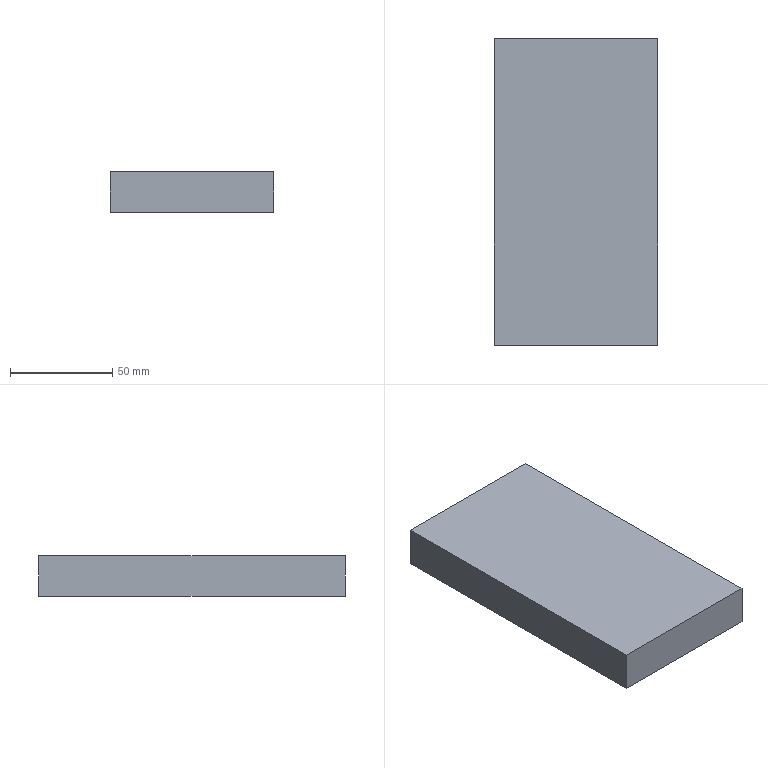Part | SolidWorks | features Extrusion 1 | 1 solid | 6 faces | box 80 x 150 x 20 mm | volume 240000 mm3 | plane 6
STEP:
#1=CARTESIAN_POINT('',(-40.,75.,0.));
#2=VERTEX_POINT('',#1);
#3=CARTESIAN_POINT('',(-40.,-75.,0.));
#4=VERTEX_POINT('',#3);
#5=CARTESIAN_POINT('',(-40.,-75.,0.));
#6=DIRECTION('',(0.,-1.,0.));
#7=VECTOR('',#6,1000.);
#8=LINE('',#5,#7);
#9=EDGE_CURVE('',#2,#4,#8,.T.);
#10=ORIENTED_EDGE('',*,*,#9,.T.);
#11=CARTESIAN_POINT('',(-40.,-75.,20.));
#12=VERTEX_POINT('',#11);
#13=CARTESIAN_POINT('',(-40.,-75.,20.));
#14=DIRECTION('',(0.,0.,-1.));
#15=VECTOR('',#14,1000.);
#16=LINE('',#13,#15);
#17=EDGE_CURVE('',#12,#4,#16,.T.);
#18=ORIENTED_EDGE('',*,*,#17,.F.);
#19=CARTESIAN_POINT('',(-40.,75.,20.));
#20=VERTEX_POINT('',#19);
#21=CARTESIAN_POINT('',(-40.,-75.,20.));
#22=DIRECTION('',(0.,-1.,0.));
#23=VECTOR('',#22,1000.);
#24=LINE('',#21,#23);
#25=EDGE_CURVE('',#20,#12,#24,.T.);
#26=ORIENTED_EDGE('',*,*,#25,.F.);
#27=CARTESIAN_POINT('',(-40.,75.,20.));
#28=DIRECTION('',(0.,0.,-1.));
#29=VECTOR('',#28,1000.);
#30=LINE('',#27,#29);
#31=EDGE_CURVE('',#20,#2,#30,.T.);
#32=ORIENTED_EDGE('',*,*,#31,.T.);
#33=EDGE_LOOP('',(#10,#18,#26,#32));
#34=FACE_OUTER_BOUND('',#33,.T.);
#35=CARTESIAN_POINT('',(-40.,-75.,20.));
#36=DIRECTION('',(1.,0.,0.));
#37=DIRECTION('',(0.,0.,-1.));
#38=AXIS2_PLACEMENT_3D('',#35,#36,#37);
#39=PLANE('',#38);
#40=ADVANCED_FACE('',(#34),#39,.F.);
#41=CARTESIAN_POINT('',(40.,-75.,0.));
#42=VERTEX_POINT('',#41);
#43=CARTESIAN_POINT('',(40.,-75.,0.));
#44=DIRECTION('',(1.,0.,0.));
#45=VECTOR('',#44,1000.);
#46=LINE('',#43,#45);
#47=EDGE_CURVE('',#4,#42,#46,.T.);
#48=ORIENTED_EDGE('',*,*,#47,.T.);
#49=CARTESIAN_POINT('',(40.,-75.,20.));
#50=VERTEX_POINT('',#49);
#51=CARTESIAN_POINT('',(40.,-75.,20.));
#52=DIRECTION('',(0.,0.,-1.));
#53=VECTOR('',#52,1000.);
#54=LINE('',#51,#53);
#55=EDGE_CURVE('',#50,#42,#54,.T.);
#56=ORIENTED_EDGE('',*,*,#55,.F.);
#57=CARTESIAN_POINT('',(40.,-75.,20.));
#58=DIRECTION('',(1.,0.,0.));
#59=VECTOR('',#58,1000.);
#60=LINE('',#57,#59);
#61=EDGE_CURVE('',#12,#50,#60,.T.);
#62=ORIENTED_EDGE('',*,*,#61,.F.);
#63=ORIENTED_EDGE('',*,*,#17,.T.);
#64=EDGE_LOOP('',(#48,#56,#62,#63));
#65=FACE_OUTER_BOUND('',#64,.T.);
#66=CARTESIAN_POINT('',(40.,-75.,20.));
#67=DIRECTION('',(0.,1.,0.));
#68=DIRECTION('',(-1.,0.,0.));
#69=AXIS2_PLACEMENT_3D('',#66,#67,#68);
#70=PLANE('',#69);
#71=ADVANCED_FACE('',(#65),#70,.F.);
#72=CARTESIAN_POINT('',(40.,75.,0.));
#73=VERTEX_POINT('',#72);
#74=CARTESIAN_POINT('',(40.,-75.,0.));
#75=DIRECTION('',(0.,1.,0.));
#76=VECTOR('',#75,1000.);
#77=LINE('',#74,#76);
#78=EDGE_CURVE('',#42,#73,#77,.T.);
#79=ORIENTED_EDGE('',*,*,#78,.T.);
#80=CARTESIAN_POINT('',(40.,75.,20.));
#81=VERTEX_POINT('',#80);
#82=CARTESIAN_POINT('',(40.,75.,20.));
#83=DIRECTION('',(0.,0.,-1.));
#84=VECTOR('',#83,1000.);
#85=LINE('',#82,#84);
#86=EDGE_CURVE('',#81,#73,#85,.T.);
#87=ORIENTED_EDGE('',*,*,#86,.F.);
#88=CARTESIAN_POINT('',(40.,-75.,20.));
#89=DIRECTION('',(0.,1.,0.));
#90=VECTOR('',#89,1000.);
#91=LINE('',#88,#90);
#92=EDGE_CURVE('',#50,#81,#91,.T.);
#93=ORIENTED_EDGE('',*,*,#92,.F.);
#94=ORIENTED_EDGE('',*,*,#55,.T.);
#95=EDGE_LOOP('',(#79,#87,#93,#94));
#96=FACE_OUTER_BOUND('',#95,.T.);
#97=CARTESIAN_POINT('',(40.,-75.,20.));
#98=DIRECTION('',(-1.,0.,0.));
#99=DIRECTION('',(0.,0.,1.));
#100=AXIS2_PLACEMENT_3D('',#97,#98,#99);
#101=PLANE('',#100);
#102=ADVANCED_FACE('',(#96),#101,.F.);
#103=CARTESIAN_POINT('',(40.,75.,0.));
#104=DIRECTION('',(-1.,0.,0.));
#105=VECTOR('',#104,1000.);
#106=LINE('',#103,#105);
#107=EDGE_CURVE('',#73,#2,#106,.T.);
#108=ORIENTED_EDGE('',*,*,#107,.T.);
#109=ORIENTED_EDGE('',*,*,#31,.F.);
#110=CARTESIAN_POINT('',(40.,75.,20.));
#111=DIRECTION('',(-1.,0.,0.));
#112=VECTOR('',#111,1000.);
#113=LINE('',#110,#112);
#114=EDGE_CURVE('',#81,#20,#113,.T.);
#115=ORIENTED_EDGE('',*,*,#114,.F.);
#116=ORIENTED_EDGE('',*,*,#86,.T.);
#117=EDGE_LOOP('',(#108,#109,#115,#116));
#118=FACE_OUTER_BOUND('',#117,.T.);
#119=CARTESIAN_POINT('',(40.,75.,20.));
#120=DIRECTION('',(0.,-1.,0.));
#121=DIRECTION('',(1.,0.,0.));
#122=AXIS2_PLACEMENT_3D('',#119,#120,#121);
#123=PLANE('',#122);
#124=ADVANCED_FACE('',(#118),#123,.F.);
#125=ORIENTED_EDGE('',*,*,#25,.T.);
#126=ORIENTED_EDGE('',*,*,#61,.T.);
#127=ORIENTED_EDGE('',*,*,#92,.T.);
#128=ORIENTED_EDGE('',*,*,#114,.T.);
#129=EDGE_LOOP('',(#125,#126,#127,#128));
#130=FACE_OUTER_BOUND('',#129,.T.);
#131=CARTESIAN_POINT('',(0.,0.,20.));
#132=DIRECTION('',(0.,0.,1.));
#133=DIRECTION('',(1.,0.,0.));
#134=AXIS2_PLACEMENT_3D('',#131,#132,#133);
#135=PLANE('',#134);
#136=ADVANCED_FACE('',(#130),#135,.T.);
#137=ORIENTED_EDGE('',*,*,#9,.F.);
#138=ORIENTED_EDGE('',*,*,#107,.F.);
#139=ORIENTED_EDGE('',*,*,#78,.F.);
#140=ORIENTED_EDGE('',*,*,#47,.F.);
#141=EDGE_LOOP('',(#137,#138,#139,#140));
#142=FACE_OUTER_BOUND('',#141,.T.);
#143=CARTESIAN_POINT('',(0.,0.,0.));
#144=DIRECTION('',(0.,0.,1.));
#145=DIRECTION('',(1.,0.,0.));
#146=AXIS2_PLACEMENT_3D('',#143,#144,#145);
#147=PLANE('',#146);
#148=ADVANCED_FACE('',(#142),#147,.F.);
#149=CLOSED_SHELL('',(#40,#71,#102,#124,#136,#148));
#150=MANIFOLD_SOLID_BREP('',#149);
#151=CARTESIAN_POINT('',(0.,0.,0.));
#152=DIRECTION('',(0.,0.,1.));
#153=DIRECTION('',(1.,0.,0.));
#154=AXIS2_PLACEMENT_3D('',#151,#152,#153);
#155=(LENGTH_UNIT()NAMED_UNIT(*)SI_UNIT(.MILLI.,.METRE.));
#156=UNCERTAINTY_MEASURE_WITH_UNIT(LENGTH_MEASURE(0.00001),#155,'','');
#157=(NAMED_UNIT(*)PLANE_ANGLE_UNIT()SI_UNIT($,.RADIAN.));
#158=(NAMED_UNIT(*)SI_UNIT($,.STERADIAN.)SOLID_ANGLE_UNIT());
#159=(GEOMETRIC_REPRESENTATION_CONTEXT(3)GLOBAL_UNCERTAINTY_ASSIGNED_CONTEXT((#156))GLOBAL_UNIT_ASSIGNED_CONTEXT((#155,#157,#158))REPRESENTATION_CONTEXT('',''));
#160=ADVANCED_BREP_SHAPE_REPRESENTATION('',(#150,#154),#159);